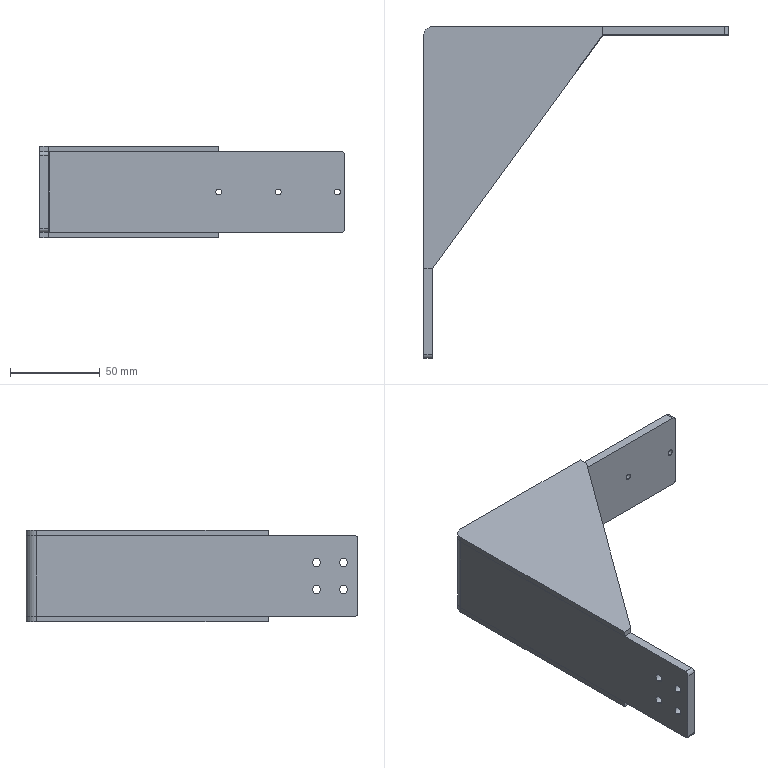Part | STEP file | PN_0001-1.5Z direct-connect drag chain fixing piece | 3 solids | 48 faces | box 170 x 185 x 51 mm | volume 121882 mm3 | plane 26 | cylinder 22 | commonest cylinder face diameters 4.5 x8 3.3 x6 4 x4 11.473 x3 1.473 x1